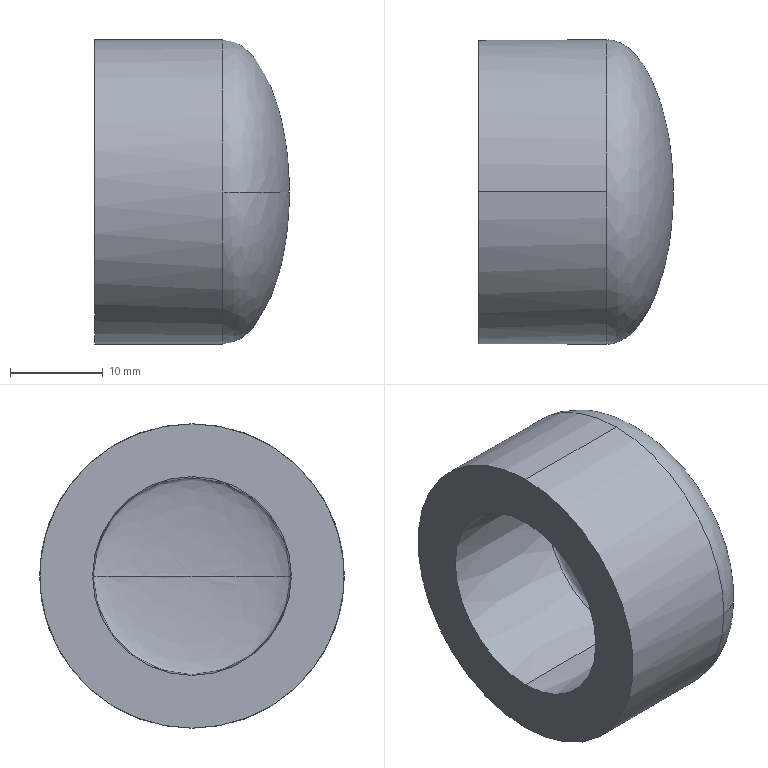Part | SolidWorks | features BaseBody 1 | 1 solid | 9 faces | box 20.956 x 32.766 x 32.766 mm | volume 10405 mm3 | spline 4 | cone 2 | cylinder 2 | plane 1 | commonest cylinder face diameters 32.766 x2
STEP:
#1=CARTESIAN_POINT('',(-5.478,0.,10.706));
#2=VERTEX_POINT('',#1);
#3=CARTESIAN_POINT('',(-5.478,0.,-10.706));
#4=VERTEX_POINT('',#3);
#5=CARTESIAN_POINT('',(-5.478,0.,0.));
#6=DIRECTION('',(-1.,0.,0.));
#7=DIRECTION('',(0.,0.,1.));
#8=AXIS2_PLACEMENT_3D('',#5,#6,#7);
#9=CIRCLE('',#8,10.706);
#10=EDGE_CURVE('',#2,#4,#9,.T.);
#11=ORIENTED_EDGE('',*,*,#10,.F.);
#12=CARTESIAN_POINT('',(-5.478,0.,0.));
#13=DIRECTION('',(-1.,0.,0.));
#14=DIRECTION('',(0.,0.,-1.));
#15=AXIS2_PLACEMENT_3D('',#12,#13,#14);
#16=CIRCLE('',#15,10.706);
#17=EDGE_CURVE('',#4,#2,#16,.T.);
#18=ORIENTED_EDGE('',*,*,#17,.F.);
#19=EDGE_LOOP('',(#11,#18));
#20=FACE_BOUND('',#19,.T.);
#21=CARTESIAN_POINT('',(-5.478,0.,16.383));
#22=VERTEX_POINT('',#21);
#23=CARTESIAN_POINT('',(-5.478,0.,-16.383));
#24=VERTEX_POINT('',#23);
#25=CARTESIAN_POINT('',(-5.478,0.,0.));
#26=DIRECTION('',(1.,0.,0.));
#27=DIRECTION('',(0.,0.,1.));
#28=AXIS2_PLACEMENT_3D('',#25,#26,#27);
#29=CIRCLE('',#28,16.383);
#30=EDGE_CURVE('',#22,#24,#29,.T.);
#31=ORIENTED_EDGE('',*,*,#30,.F.);
#32=CARTESIAN_POINT('',(-5.478,0.,0.));
#33=DIRECTION('',(1.,0.,0.));
#34=DIRECTION('',(0.,0.,-1.));
#35=AXIS2_PLACEMENT_3D('',#32,#33,#34);
#36=CIRCLE('',#35,16.383);
#37=EDGE_CURVE('',#24,#22,#36,.T.);
#38=ORIENTED_EDGE('',*,*,#37,.F.);
#39=EDGE_LOOP('',(#31,#38));
#40=FACE_OUTER_BOUND('',#39,.T.);
#41=CARTESIAN_POINT('',(-5.478,-16.383,0.));
#42=DIRECTION('',(-1.,0.,0.));
#43=DIRECTION('',(0.,0.,1.));
#44=AXIS2_PLACEMENT_3D('',#41,#42,#43);
#45=PLANE('',#44);
#46=ADVANCED_FACE('',(#20,#40),#45,.T.);
#47=CARTESIAN_POINT('',(9.712,0.,0.));
#48=VERTEX_POINT('',#47);
#49=CARTESIAN_POINT('',(8.334,10.617,0.));
#50=VERTEX_POINT('',#49);
#51=CARTESIAN_POINT('',(9.712,0.,0.));
#52=CARTESIAN_POINT('',(9.712,6.219,0.));
#53=CARTESIAN_POINT('',(9.142,10.617,0.));
#54=CARTESIAN_POINT('',(8.334,10.617,0.));
#55=(BOUNDED_CURVE()B_SPLINE_CURVE(3,(#51,#52,#53,#54),.UNSPECIFIED.,.F.,.F.)B_SPLINE_CURVE_WITH_KNOTS((4,4),(1.571,3.142),.UNSPECIFIED.)CURVE()GEOMETRIC_REPRESENTATION_ITEM()RATIONAL_B_SPLINE_CURVE((1.,0.8047,0.8047,1.))REPRESENTATION_ITEM(''));
#56=EDGE_CURVE('',#48,#50,#55,.T.);
#57=ORIENTED_EDGE('',*,*,#56,.F.);
#58=CARTESIAN_POINT('',(8.334,-10.617,0.));
#59=VERTEX_POINT('',#58);
#60=CARTESIAN_POINT('',(8.334,-10.617,0.));
#61=CARTESIAN_POINT('',(9.142,-10.617,0.));
#62=CARTESIAN_POINT('',(9.712,-6.219,0.));
#63=CARTESIAN_POINT('',(9.712,0.,0.));
#64=(BOUNDED_CURVE()B_SPLINE_CURVE(3,(#60,#61,#62,#63),.UNSPECIFIED.,.F.,.F.)B_SPLINE_CURVE_WITH_KNOTS((4,4),(0.,1.571),.UNSPECIFIED.)CURVE()GEOMETRIC_REPRESENTATION_ITEM()RATIONAL_B_SPLINE_CURVE((1.,0.8047,0.8047,1.))REPRESENTATION_ITEM(''));
#65=EDGE_CURVE('',#59,#48,#64,.T.);
#66=ORIENTED_EDGE('',*,*,#65,.F.);
#67=CARTESIAN_POINT('',(8.334,0.,10.617));
#68=VERTEX_POINT('',#67);
#69=CARTESIAN_POINT('',(8.334,0.,0.));
#70=DIRECTION('',(1.,0.,0.));
#71=DIRECTION('',(0.,0.,1.));
#72=AXIS2_PLACEMENT_3D('',#69,#70,#71);
#73=CIRCLE('',#72,10.617);
#74=EDGE_CURVE('',#68,#59,#73,.T.);
#75=ORIENTED_EDGE('',*,*,#74,.F.);
#76=CARTESIAN_POINT('',(8.334,0.,0.));
#77=DIRECTION('',(1.,0.,0.));
#78=DIRECTION('',(0.,1.,0.));
#79=AXIS2_PLACEMENT_3D('',#76,#77,#78);
#80=CIRCLE('',#79,10.617);
#81=EDGE_CURVE('',#50,#68,#80,.T.);
#82=ORIENTED_EDGE('',*,*,#81,.F.);
#83=EDGE_LOOP('',(#57,#66,#75,#82));
#84=FACE_OUTER_BOUND('',#83,.T.);
#85=CARTESIAN_POINT('',(9.712,0.,0.));
#86=CARTESIAN_POINT('',(9.712,0.,0.));
#87=CARTESIAN_POINT('',(9.712,0.,0.));
#88=CARTESIAN_POINT('',(9.712,0.,0.));
#89=CARTESIAN_POINT('',(9.712,-6.219,0.));
#90=CARTESIAN_POINT('',(9.712,-6.219,12.439));
#91=CARTESIAN_POINT('',(9.712,6.219,12.439));
#92=CARTESIAN_POINT('',(9.712,6.219,0.));
#93=CARTESIAN_POINT('',(9.142,-10.617,0.));
#94=CARTESIAN_POINT('',(9.142,-10.617,21.234));
#95=CARTESIAN_POINT('',(9.142,10.617,21.234));
#96=CARTESIAN_POINT('',(9.142,10.617,0.));
#97=CARTESIAN_POINT('',(8.334,-10.617,0.));
#98=CARTESIAN_POINT('',(8.334,-10.617,21.234));
#99=CARTESIAN_POINT('',(8.334,10.617,21.234));
#100=CARTESIAN_POINT('',(8.334,10.617,0.));
#101=(BOUNDED_SURFACE()B_SPLINE_SURFACE(3,3,((#85,#86,#87,#88),(#89,#90,#91,#92),(#93,#94,#95,#96),(#97,#98,#99,#100)),.UNSPECIFIED.,.F.,.F.,.F.)B_SPLINE_SURFACE_WITH_KNOTS((4,4),(4,4),(0.,1.),(0.,1.),.UNSPECIFIED.)GEOMETRIC_REPRESENTATION_ITEM()RATIONAL_B_SPLINE_SURFACE(((1.,0.3333,0.3333,1.),(0.8047,0.2682,0.2682,0.8047),(0.8047,0.2682,0.2682,0.8047),(1.,0.3333,0.3333,1.)))REPRESENTATION_ITEM('')SURFACE());
#102=ADVANCED_FACE('',(#84),#101,.T.);
#103=CARTESIAN_POINT('',(8.334,16.383,0.));
#104=VERTEX_POINT('',#103);
#105=CARTESIAN_POINT('',(15.478,0.,0.));
#106=VERTEX_POINT('',#105);
#107=CARTESIAN_POINT('',(8.334,16.383,0.));
#108=CARTESIAN_POINT('',(12.519,16.383,0.));
#109=CARTESIAN_POINT('',(15.478,9.597,0.));
#110=CARTESIAN_POINT('',(15.478,0.,0.));
#111=(BOUNDED_CURVE()B_SPLINE_CURVE(3,(#107,#108,#109,#110),.UNSPECIFIED.,.F.,.F.)B_SPLINE_CURVE_WITH_KNOTS((4,4),(0.,1.571),.UNSPECIFIED.)CURVE()GEOMETRIC_REPRESENTATION_ITEM()RATIONAL_B_SPLINE_CURVE((1.,0.8047,0.8047,1.))REPRESENTATION_ITEM(''));
#112=EDGE_CURVE('',#104,#106,#111,.T.);
#113=ORIENTED_EDGE('',*,*,#112,.F.);
#114=CARTESIAN_POINT('',(8.334,0.,16.383));
#115=VERTEX_POINT('',#114);
#116=CARTESIAN_POINT('',(8.334,0.,0.));
#117=DIRECTION('',(-1.,0.,0.));
#118=DIRECTION('',(0.,0.,1.));
#119=AXIS2_PLACEMENT_3D('',#116,#117,#118);
#120=CIRCLE('',#119,16.383);
#121=EDGE_CURVE('',#115,#104,#120,.T.);
#122=ORIENTED_EDGE('',*,*,#121,.F.);
#123=CARTESIAN_POINT('',(8.334,-16.383,0.));
#124=VERTEX_POINT('',#123);
#125=CARTESIAN_POINT('',(8.334,0.,0.));
#126=DIRECTION('',(-1.,0.,0.));
#127=DIRECTION('',(0.,-1.,0.));
#128=AXIS2_PLACEMENT_3D('',#125,#126,#127);
#129=CIRCLE('',#128,16.383);
#130=EDGE_CURVE('',#124,#115,#129,.T.);
#131=ORIENTED_EDGE('',*,*,#130,.F.);
#132=CARTESIAN_POINT('',(15.478,0.,0.));
#133=CARTESIAN_POINT('',(15.478,-9.597,0.));
#134=CARTESIAN_POINT('',(12.519,-16.383,0.));
#135=CARTESIAN_POINT('',(8.334,-16.383,0.));
#136=(BOUNDED_CURVE()B_SPLINE_CURVE(3,(#132,#133,#134,#135),.UNSPECIFIED.,.F.,.T.)B_SPLINE_CURVE_WITH_KNOTS((4,4),(1.571,3.142),.UNSPECIFIED.)CURVE()GEOMETRIC_REPRESENTATION_ITEM()RATIONAL_B_SPLINE_CURVE((1.,0.8047,0.8047,1.))REPRESENTATION_ITEM(''));
#137=EDGE_CURVE('',#106,#124,#136,.T.);
#138=ORIENTED_EDGE('',*,*,#137,.F.);
#139=EDGE_LOOP('',(#113,#122,#131,#138));
#140=FACE_OUTER_BOUND('',#139,.T.);
#141=CARTESIAN_POINT('',(8.334,-16.383,0.));
#142=CARTESIAN_POINT('',(8.334,-16.383,32.766));
#143=CARTESIAN_POINT('',(8.334,16.383,32.766));
#144=CARTESIAN_POINT('',(8.334,16.383,0.));
#145=CARTESIAN_POINT('',(12.519,-16.383,0.));
#146=CARTESIAN_POINT('',(12.519,-16.383,32.766));
#147=CARTESIAN_POINT('',(12.519,16.383,32.766));
#148=CARTESIAN_POINT('',(12.519,16.383,0.));
#149=CARTESIAN_POINT('',(15.478,-9.597,0.));
#150=CARTESIAN_POINT('',(15.478,-9.597,19.194));
#151=CARTESIAN_POINT('',(15.478,9.597,19.194));
#152=CARTESIAN_POINT('',(15.478,9.597,0.));
#153=CARTESIAN_POINT('',(15.478,0.,0.));
#154=CARTESIAN_POINT('',(15.478,0.,0.));
#155=CARTESIAN_POINT('',(15.478,0.,0.));
#156=CARTESIAN_POINT('',(15.478,0.,0.));
#157=(BOUNDED_SURFACE()B_SPLINE_SURFACE(3,3,((#141,#142,#143,#144),(#145,#146,#147,#148),(#149,#150,#151,#152),(#153,#154,#155,#156)),.UNSPECIFIED.,.F.,.F.,.T.)B_SPLINE_SURFACE_WITH_KNOTS((4,4),(4,4),(0.,1.),(0.,1.),.UNSPECIFIED.)GEOMETRIC_REPRESENTATION_ITEM()RATIONAL_B_SPLINE_SURFACE(((1.,0.3333,0.3333,1.),(0.8047,0.2682,0.2682,0.8047),(0.8047,0.2682,0.2682,0.8047),(1.,0.3333,0.3333,1.)))REPRESENTATION_ITEM('')SURFACE());
#158=ADVANCED_FACE('',(#140),#157,.T.);
#159=ORIENTED_EDGE('',*,*,#81,.T.);
#160=CARTESIAN_POINT('',(-5.478,0.,10.706));
#161=DIRECTION('',(1.,0.,-0.0064));
#162=VECTOR('',#161,1000.);
#163=LINE('',#160,#162);
#164=EDGE_CURVE('',#2,#68,#163,.T.);
#165=ORIENTED_EDGE('',*,*,#164,.F.);
#166=ORIENTED_EDGE('',*,*,#10,.T.);
#167=CARTESIAN_POINT('',(8.334,0.,-10.617));
#168=VERTEX_POINT('',#167);
#169=CARTESIAN_POINT('',(8.334,0.,-10.617));
#170=DIRECTION('',(-1.,0.,-0.0064));
#171=VECTOR('',#170,1000.);
#172=LINE('',#169,#171);
#173=EDGE_CURVE('',#168,#4,#172,.T.);
#174=ORIENTED_EDGE('',*,*,#173,.F.);
#175=CARTESIAN_POINT('',(8.334,0.,0.));
#176=DIRECTION('',(-1.,0.,0.));
#177=DIRECTION('',(0.,1.,0.));
#178=AXIS2_PLACEMENT_3D('',#175,#176,#177);
#179=CIRCLE('',#178,10.617);
#180=EDGE_CURVE('',#50,#168,#179,.T.);
#181=ORIENTED_EDGE('',*,*,#180,.F.);
#182=EDGE_LOOP('',(#159,#165,#166,#174,#181));
#183=FACE_OUTER_BOUND('',#182,.T.);
#184=CARTESIAN_POINT('',(48.522,0.,0.));
#185=DIRECTION('',(-1.,0.,0.));
#186=DIRECTION('',(0.,0.,1.));
#187=AXIS2_PLACEMENT_3D('',#184,#185,#186);
#188=CONICAL_SURFACE('',#187,10.36,0.0064);
#189=ADVANCED_FACE('',(#183),#188,.F.);
#190=CARTESIAN_POINT('',(8.334,0.,0.));
#191=DIRECTION('',(-1.,0.,0.));
#192=DIRECTION('',(0.,0.,-1.));
#193=AXIS2_PLACEMENT_3D('',#190,#191,#192);
#194=CIRCLE('',#193,10.617);
#195=EDGE_CURVE('',#168,#59,#194,.T.);
#196=ORIENTED_EDGE('',*,*,#195,.F.);
#197=ORIENTED_EDGE('',*,*,#173,.T.);
#198=ORIENTED_EDGE('',*,*,#17,.T.);
#199=ORIENTED_EDGE('',*,*,#164,.T.);
#200=ORIENTED_EDGE('',*,*,#74,.T.);
#201=EDGE_LOOP('',(#196,#197,#198,#199,#200));
#202=FACE_OUTER_BOUND('',#201,.T.);
#203=CARTESIAN_POINT('',(48.522,0.,0.));
#204=DIRECTION('',(-1.,0.,0.));
#205=DIRECTION('',(0.,0.,1.));
#206=AXIS2_PLACEMENT_3D('',#203,#204,#205);
#207=CONICAL_SURFACE('',#206,10.36,0.0064);
#208=ADVANCED_FACE('',(#202),#207,.F.);
#209=ORIENTED_EDGE('',*,*,#37,.T.);
#210=CARTESIAN_POINT('',(8.334,0.,16.383));
#211=DIRECTION('',(-1.,0.,0.));
#212=VECTOR('',#211,1000.);
#213=LINE('',#210,#212);
#214=EDGE_CURVE('',#115,#22,#213,.T.);
#215=ORIENTED_EDGE('',*,*,#214,.F.);
#216=ORIENTED_EDGE('',*,*,#121,.T.);
#217=CARTESIAN_POINT('',(8.334,0.,-16.383));
#218=VERTEX_POINT('',#217);
#219=CARTESIAN_POINT('',(8.334,0.,0.));
#220=DIRECTION('',(1.,0.,0.));
#221=DIRECTION('',(0.,0.,-1.));
#222=AXIS2_PLACEMENT_3D('',#219,#220,#221);
#223=CIRCLE('',#222,16.383);
#224=EDGE_CURVE('',#218,#104,#223,.T.);
#225=ORIENTED_EDGE('',*,*,#224,.F.);
#226=CARTESIAN_POINT('',(-5.478,0.,-16.383));
#227=DIRECTION('',(1.,0.,0.));
#228=VECTOR('',#227,1000.);
#229=LINE('',#226,#228);
#230=EDGE_CURVE('',#24,#218,#229,.T.);
#231=ORIENTED_EDGE('',*,*,#230,.F.);
#232=EDGE_LOOP('',(#209,#215,#216,#225,#231));
#233=FACE_OUTER_BOUND('',#232,.T.);
#234=CARTESIAN_POINT('',(8.334,0.,0.));
#235=DIRECTION('',(-1.,0.,0.));
#236=DIRECTION('',(0.,0.,1.));
#237=AXIS2_PLACEMENT_3D('',#234,#235,#236);
#238=CYLINDRICAL_SURFACE('',#237,16.383);
#239=ADVANCED_FACE('',(#233),#238,.T.);
#240=ORIENTED_EDGE('',*,*,#230,.T.);
#241=CARTESIAN_POINT('',(8.334,0.,0.));
#242=DIRECTION('',(1.,0.,0.));
#243=DIRECTION('',(0.,-1.,0.));
#244=AXIS2_PLACEMENT_3D('',#241,#242,#243);
#245=CIRCLE('',#244,16.383);
#246=EDGE_CURVE('',#124,#218,#245,.T.);
#247=ORIENTED_EDGE('',*,*,#246,.F.);
#248=ORIENTED_EDGE('',*,*,#130,.T.);
#249=ORIENTED_EDGE('',*,*,#214,.T.);
#250=ORIENTED_EDGE('',*,*,#30,.T.);
#251=EDGE_LOOP('',(#240,#247,#248,#249,#250));
#252=FACE_OUTER_BOUND('',#251,.T.);
#253=CARTESIAN_POINT('',(8.334,0.,0.));
#254=DIRECTION('',(-1.,0.,0.));
#255=DIRECTION('',(0.,0.,1.));
#256=AXIS2_PLACEMENT_3D('',#253,#254,#255);
#257=CYLINDRICAL_SURFACE('',#256,16.383);
#258=ADVANCED_FACE('',(#252),#257,.T.);
#259=ORIENTED_EDGE('',*,*,#224,.T.);
#260=ORIENTED_EDGE('',*,*,#112,.T.);
#261=ORIENTED_EDGE('',*,*,#137,.T.);
#262=ORIENTED_EDGE('',*,*,#246,.T.);
#263=EDGE_LOOP('',(#259,#260,#261,#262));
#264=FACE_OUTER_BOUND('',#263,.T.);
#265=CARTESIAN_POINT('',(8.334,16.383,0.));
#266=CARTESIAN_POINT('',(8.334,16.383,-32.766));
#267=CARTESIAN_POINT('',(8.334,-16.383,-32.766));
#268=CARTESIAN_POINT('',(8.334,-16.383,0.));
#269=CARTESIAN_POINT('',(12.519,16.383,0.));
#270=CARTESIAN_POINT('',(12.519,16.383,-32.766));
#271=CARTESIAN_POINT('',(12.519,-16.383,-32.766));
#272=CARTESIAN_POINT('',(12.519,-16.383,0.));
#273=CARTESIAN_POINT('',(15.478,9.597,0.));
#274=CARTESIAN_POINT('',(15.478,9.597,-19.194));
#275=CARTESIAN_POINT('',(15.478,-9.597,-19.194));
#276=CARTESIAN_POINT('',(15.478,-9.597,0.));
#277=CARTESIAN_POINT('',(15.478,0.,0.));
#278=CARTESIAN_POINT('',(15.478,0.,0.));
#279=CARTESIAN_POINT('',(15.478,0.,0.));
#280=CARTESIAN_POINT('',(15.478,0.,0.));
#281=(BOUNDED_SURFACE()B_SPLINE_SURFACE(3,3,((#265,#266,#267,#268),(#269,#270,#271,#272),(#273,#274,#275,#276),(#277,#278,#279,#280)),.UNSPECIFIED.,.F.,.F.,.F.)B_SPLINE_SURFACE_WITH_KNOTS((4,4),(4,4),(0.,1.),(0.,1.),.UNSPECIFIED.)GEOMETRIC_REPRESENTATION_ITEM()RATIONAL_B_SPLINE_SURFACE(((1.,0.3333,0.3333,1.),(0.8047,0.2682,0.2682,0.8047),(0.8047,0.2682,0.2682,0.8047),(1.,0.3333,0.3333,1.)))REPRESENTATION_ITEM('')SURFACE());
#282=ADVANCED_FACE('',(#264),#281,.T.);
#283=ORIENTED_EDGE('',*,*,#65,.T.);
#284=ORIENTED_EDGE('',*,*,#56,.T.);
#285=ORIENTED_EDGE('',*,*,#180,.T.);
#286=ORIENTED_EDGE('',*,*,#195,.T.);
#287=EDGE_LOOP('',(#283,#284,#285,#286));
#288=FACE_OUTER_BOUND('',#287,.T.);
#289=CARTESIAN_POINT('',(9.712,0.,0.));
#290=CARTESIAN_POINT('',(9.712,0.,0.));
#291=CARTESIAN_POINT('',(9.712,0.,0.));
#292=CARTESIAN_POINT('',(9.712,0.,0.));
#293=CARTESIAN_POINT('',(9.712,6.219,0.));
#294=CARTESIAN_POINT('',(9.712,6.219,-12.439));
#295=CARTESIAN_POINT('',(9.712,-6.219,-12.439));
#296=CARTESIAN_POINT('',(9.712,-6.219,0.));
#297=CARTESIAN_POINT('',(9.142,10.617,0.));
#298=CARTESIAN_POINT('',(9.142,10.617,-21.234));
#299=CARTESIAN_POINT('',(9.142,-10.617,-21.234));
#300=CARTESIAN_POINT('',(9.142,-10.617,0.));
#301=CARTESIAN_POINT('',(8.334,10.617,0.));
#302=CARTESIAN_POINT('',(8.334,10.617,-21.234));
#303=CARTESIAN_POINT('',(8.334,-10.617,-21.234));
#304=CARTESIAN_POINT('',(8.334,-10.617,0.));
#305=(BOUNDED_SURFACE()B_SPLINE_SURFACE(3,3,((#289,#290,#291,#292),(#293,#294,#295,#296),(#297,#298,#299,#300),(#301,#302,#303,#304)),.UNSPECIFIED.,.F.,.F.,.F.)B_SPLINE_SURFACE_WITH_KNOTS((4,4),(4,4),(0.,1.),(0.,1.),.UNSPECIFIED.)GEOMETRIC_REPRESENTATION_ITEM()RATIONAL_B_SPLINE_SURFACE(((1.,0.3333,0.3333,1.),(0.8047,0.2682,0.2682,0.8047),(0.8047,0.2682,0.2682,0.8047),(1.,0.3333,0.3333,1.)))REPRESENTATION_ITEM('')SURFACE());
#306=ADVANCED_FACE('',(#288),#305,.T.);
#307=CLOSED_SHELL('',(#46,#102,#158,#189,#208,#239,#258,#282,#306));
#308=MANIFOLD_SOLID_BREP('',#307);
#309=CARTESIAN_POINT('',(0.,0.,0.));
#310=DIRECTION('',(0.,0.,1.));
#311=DIRECTION('',(1.,0.,0.));
#312=AXIS2_PLACEMENT_3D('',#309,#310,#311);
#313=(LENGTH_UNIT()NAMED_UNIT(*)SI_UNIT(.MILLI.,.METRE.));
#314=UNCERTAINTY_MEASURE_WITH_UNIT(LENGTH_MEASURE(0.00001),#313,'','');
#315=(NAMED_UNIT(*)PLANE_ANGLE_UNIT()SI_UNIT($,.RADIAN.));
#316=(NAMED_UNIT(*)SI_UNIT($,.STERADIAN.)SOLID_ANGLE_UNIT());
#317=(GEOMETRIC_REPRESENTATION_CONTEXT(3)GLOBAL_UNCERTAINTY_ASSIGNED_CONTEXT((#314))GLOBAL_UNIT_ASSIGNED_CONTEXT((#313,#315,#316))REPRESENTATION_CONTEXT('',''));
#318=ADVANCED_BREP_SHAPE_REPRESENTATION('',(#308,#312),#317);